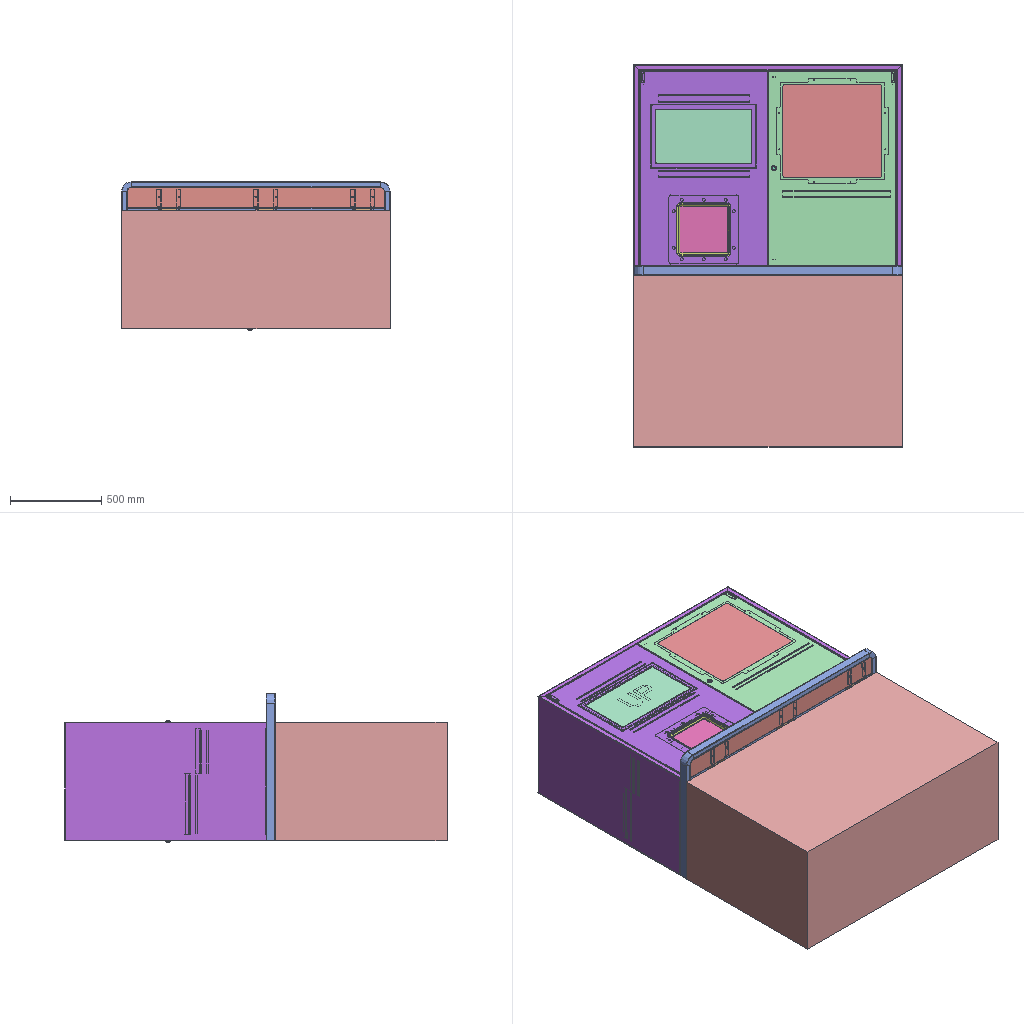Assembly | SolidWorks | 122 different items | 247 placed | box 1470 x 2090 x 812 mm
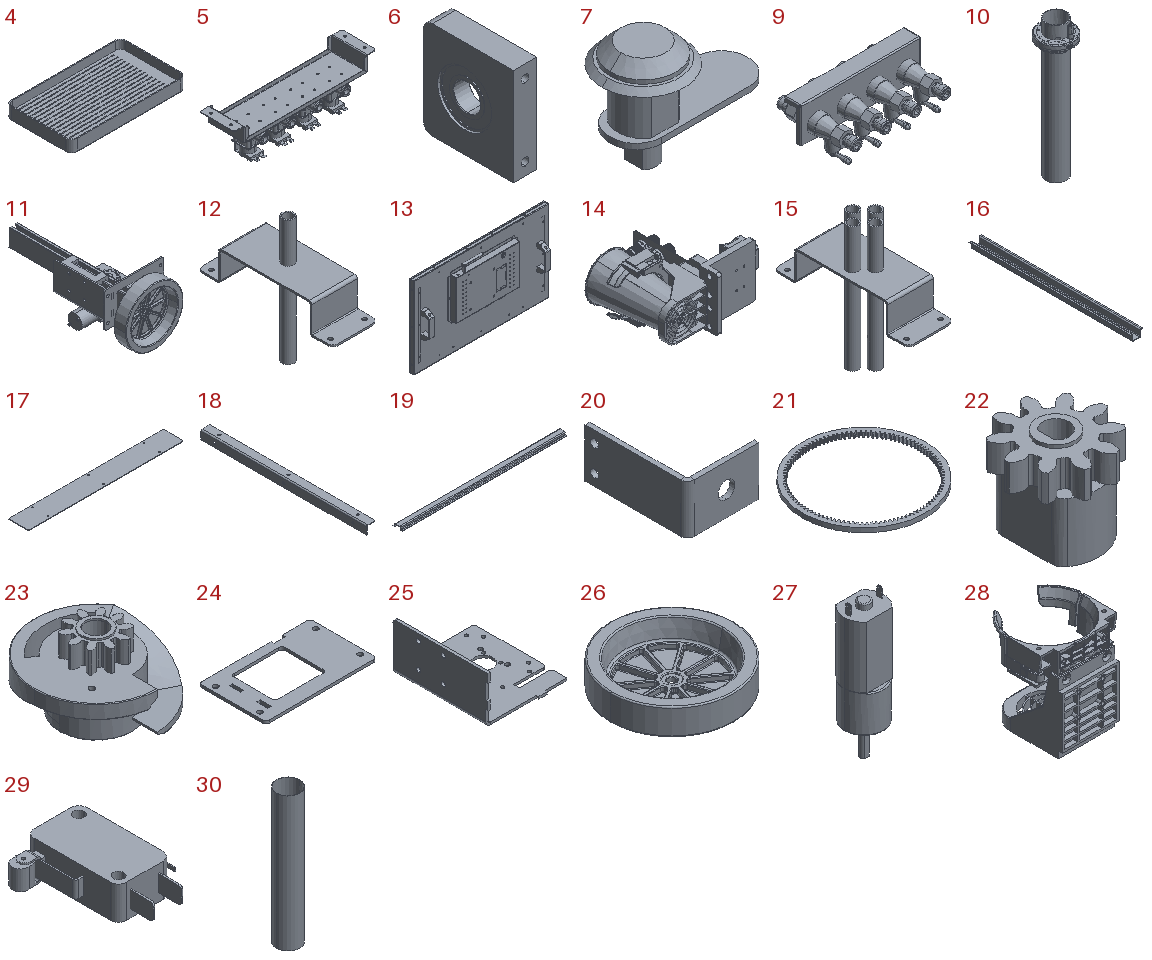Parts list (item | name | quantity | parent item | size | volume | features):
1 | 90 Capper Limit Switch Adjustable Bracket | x1 | - | - | - | -
2 | 90 mm Bore 5840-42 Rotary Capper Motor | x1 | - | - | - | -
3 | 90 mm Capper Limit Switch | x1 | - | - | - | -
4 | (subassembly) | x1 | - | 390 x 225 x 48 mm | 613615 mm3 | features AEMSimFeature 1
5 | (subassembly) | x1 | - | 287.6 x 73.8 x 84.7 mm | 205450 mm3 | features ReferencePattern 3, AEMSimFeature 1, LocalLPattern 1
6 | (subassembly) | x2 | in 14 | 13 x 50 x 54 mm | 29631 mm3 | features AEMSimFeature 1
7 | (subassembly) | x2 | - | 53.001 x 30 x 37.4 mm | 9862 mm3 | features AEMSimFeature 1
8 | (subassembly) | x1 | - | - | - | features AEMSimFeature 1
9 | (subassembly) | x1 | - | 222.4 x 141.4 x 82.578 mm | 275099 mm3 | features ReferencePattern 3, AEMSimFeature 1, LocalLPattern 1
10 | (subassembly) | x4 | - | - | 425730 mm3 | features InContextFeatHolder 5, ReferencePattern 4, LocalCirPattern 1
11 | (subassembly) | x1 | - | 115 x 241 x 107.2 mm | 279061 mm3 | features InContextFeatHolder 17
12 | (subassembly) | x1 | - | 40 x 119 x 110 mm | 12883 mm3 | features AEMSimFeature 1
13 | (subassembly) | x1 | - | 580.3 x 59 x 351.2 mm | 2110380 mm3 | features AEMSimFeature 1
14 | (subassembly) | x1 | in 8 | 224.692 x 193 x 105 mm | 423865 mm3 | features ReferencePattern 3, AEMSimFeature 1, InContextFeatHolder 1, LocalLPattern 1
15 | (subassembly) | x1 | - | 40 x 119 x 110 mm | 21860 mm3 | features LocalLPattern 2, ReferencePattern 2, AEMSimFeature 1
16 | - | x2 | - | 40 x 500 x 21 mm | 56565 mm3 | features 3DProfileFeature 1, FlatPattern 1, HoleWzd 1, ICE 1, SMBaseFlange 1, SheetMetal 1
17 | - | x2 | - | 500 x 65 x 1.5 mm | 48608 mm3 | features Fillet 1, FlatPattern 1, ICE 1, LPattern 1, SMBaseFlange 1, SheetMetal 1
18 | - | x2 | - | 30 x 575 x 30 mm | 64402 mm3 | features 3DProfileFeature 2, Fillet 2, HoleWzd 2, FlatPattern 1, ICE 1, LPattern 1, SMBaseFlange 1, SheetMetal 1
19 | - | x5 | - | 590 x 34 x 10.7 mm | 34971 mm3 | features EdgeFlange 2, FlatPattern 1, SMBaseFlange 1, SheetMetal 1
20 | - | x4 | - | 22 x 31.5 x 15 mm | 1109 mm3 | features ICE 2, FlatPattern 1, SMBaseFlange 1, SheetMetal 1
21 | - | x4 | in 10 | 144.5 x 144.5 x 5.2 mm | 14739 mm3 | features CirPattern 1, Extrusion 1, ICE 1, RefAxis 1
22 | - | x4 | in 10 | 15 x 14.473 x 13.6 mm | 1407 mm3 | features ICE 5, CirPattern 1, Extrusion 1, Fillet 1, RefAxis 1
23 | - | x20 | in 10 | 34.7 x 34.7 x 20.5 mm | 6291 mm3 | features ICE 12, Chamfer 4, Fillet 4, CirPattern 2, Helix 2, SweepCut 2, Extrusion 1, RefAxis 1
24 | - | x1 | in 11 | 100 x 60 x 2.5 mm | 10028 mm3 | features Cut 2, Fillet 2, ICE 2, MirrorPattern 2, FlatPattern 1, LPattern 1, SMBaseFlange 1, SheetMetal 1
25 | - | x1 | in 11 | 85 x 99.5 x 50 mm | 30184 mm3 | features Cut 4, Fillet 2, ICE 2, EdgeFlange 1, FlatPattern 1, LPattern 1, SMBaseFlange 1, SheetMetal 1
26 | - | x1 | in 11 | 98 x 98 x 21 mm | 76167 mm3 | features ICE 6, Fillet 5, Chamfer 2, CirPattern 1, Extrusion 1
27 | - | x4 | in 10 | 20.5 x 20 x 71.9 mm | 15341 mm3 | features ICE 8, Fillet 4, MirrorPattern 3, Extrusion 1
28 | - | x1 | in 14 | 95.114 x 93.076 x 111.7 mm | 101033 mm3 | features MBimport 1
29 | - | x4 | in 10 | 27.9 x 35 x 10 mm | 4554 mm3 | features ICE 3, BaseBody 1
30 | - | x4 | in 10 | 97 x 97 x 558.5 mm | 201706 mm3 | features Extrusion 1
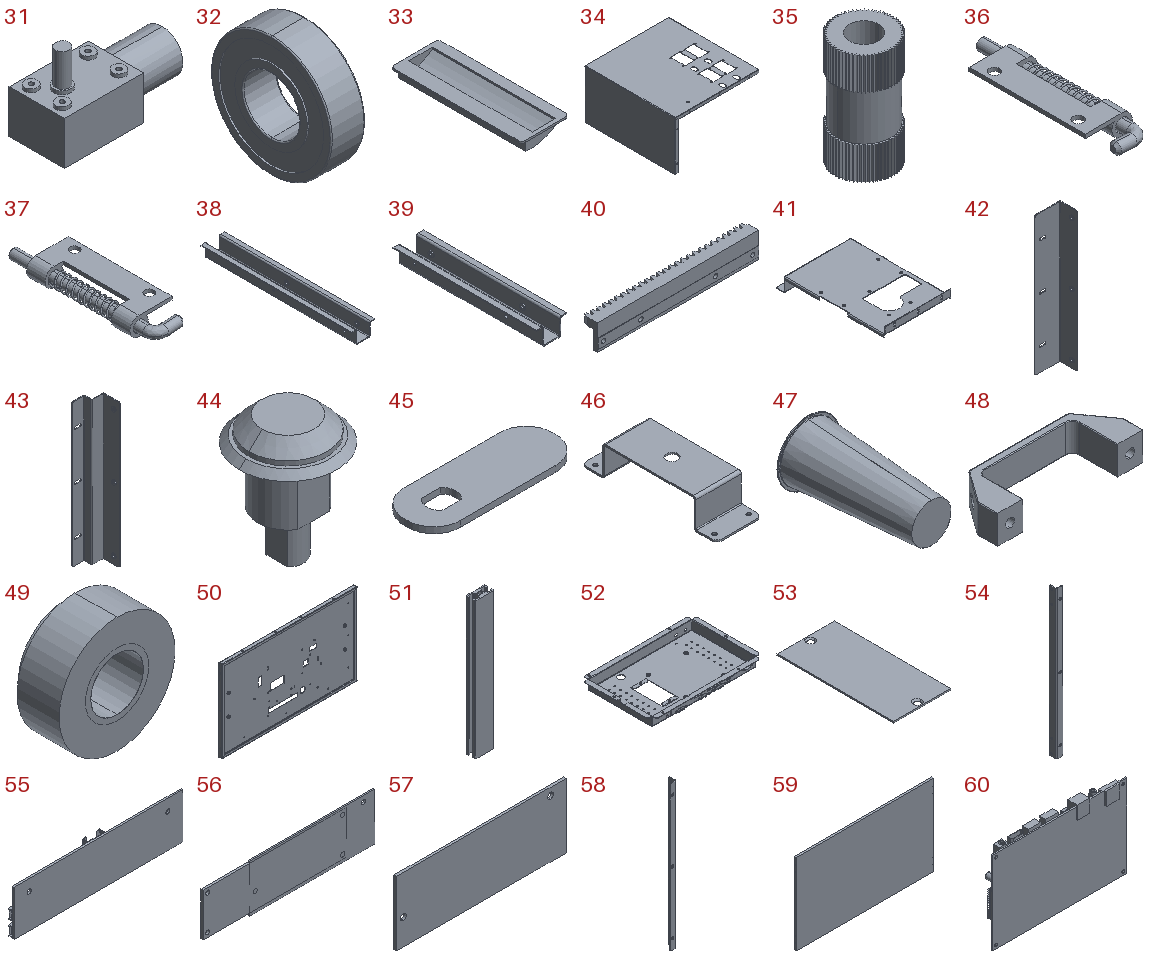31 | - | x1 | in 11 | 81 x 32 x 47.2 mm | 52588 mm3 | features ICE 7, Extrusion 1
32 | - | x2 | in 6 | 9 x 32 x 32 mm | 5366 mm3 | features BaseBody 1
33 | - | x2 | - | 40 x 110 x 10.429 mm | 7857 mm3 | features ICE 3, Extrusion 1, Fillet 1, MirrorPattern 1
34 | - | x1 | - | 568 x 611 x 333 mm | 859533 mm3 | features LPattern 4, ICE 3, Cut 2, EdgeFlange 2, 3DProfileFeature 1, FlatPattern 1, HoleWzd 1, SMBaseFlange 1, SheetMetal 1
35 | - | x16 | in 10 | 6.299 x 6.297 x 12 mm | 240.496 mm3 | features ICE 2, CirPattern 1, Extrusion 1
36 | - | x3 | - | 25.4 x 89 x 11 mm | 6004 mm3 | features MirrorStock 1
37 | - | x3 | - | 25.4 x 89 x 11 mm | 6004 mm3 | features BaseBody 3
38 | - | x2 | - | 50 x 320 x 28.5 mm | 48347 mm3 | features ICE 2, 3DProfileFeature 1, FlatPattern 1, HoleWzd 1, MirrorPattern 1, SMBaseFlange 1, SheetMetal 1
39 | - | x2 | - | 50 x 235 x 28.5 mm | 35580 mm3 | features ICE 2, 3DProfileFeature 1, FlatPattern 1, HoleWzd 1, MirrorPattern 1, SMBaseFlange 1, SheetMetal 1
40 | - | x1 | in 11 | 169.646 x 15.5 x 27 mm | 32516 mm3 | features ICE 4, LPattern 3, Boss 1, Chamfer 1, Extrusion 1, Fillet 1
41 | - | x1 | - | 236 x 382 x 73.5 mm | 191072 mm3 | features ICE 7, EdgeFlange 4, Fillet 2, SMBaseFlange 2, FlatPattern 1, MirrorPattern 1, SheetMetal 1
42 | - | x1 | - | 50 x 35 x 270 mm | 33491 mm3 | features ICE 2, 3DProfileFeature 1, Fillet 1, FlatPattern 1, HoleWzd 1, SMBaseFlange 1, SheetMetal 1
43 | - | x1 | - | 45 x 47 x 270 mm | 35809 mm3 | features ICE 2, 3DProfileFeature 1, Fillet 1, FlatPattern 1, HoleWzd 1, SMBaseFlange 1, SheetMetal 1
44 | - | x2 | in 7 | 30 x 30 x 37.4 mm | 8223 mm3 | features ICE 3, Chamfer 2, Extrusion 1
45 | - | x2 | in 7 | 50 x 19 x 2 mm | 1640 mm3 | features Fillet 1, FlatPattern 1, ICE 1, SMBaseFlange 1, SheetMetal 1
46 | - | x1 | in 12 | 40 x 119 x 26.5 mm | 9773 mm3 | features EdgeFlange 2, ICE 2, Fillet 1, FlatPattern 1, LPattern 1, SMBaseFlange 1, SheetMetal 1
47 | - | x1 | in 14 | 89 x 177.3 x 89 mm | 12581 mm3 | features RefAxis 1, Revolution 1
48 | - | x2 | in 13 | 107.5 x 38 x 21 mm | 27579 mm3 | features BaseBody 1
49 | - | x1 | in 13 | - | - | features BaseBody 1, RefSurface 1
50 | - | x1 | in 13 | - | - | features BaseBody 13, RefSurface 1
51 | - | x1 | in 11 | 30 x 15 x 220 mm | 49057 mm3 | features ICE 4, Fillet 2, MirrorPattern 2, Cut 1, Extrusion 1, LPattern 1
52 | - | x1 | in 13 | - | - | features RefSurface 13, BaseBody 12
53 | - | x1 | in 13 | 41 x 84 x 1 mm | 3404 mm3 | features BaseBody 1
54 | - | x1 | in 13 | 12 x 14.1 x 280 mm | 6830 mm3 | features BaseBody 1
55 | - | x1 | in 13 | 134 x 11.5 x 36 mm | 18226 mm3 | features BaseBody 1
56 | - | x1 | in 13 | 119.5 x 1.6 x 33.1 mm | 8199 mm3 | features BaseBody 2
57 | - | x1 | in 13 | 87 x 1.2 x 33.1 mm | 3439 mm3 | features BaseBody 1
58 | - | x1 | in 13 | 12 x 14.1 x 280 mm | 6824 mm3 | features BaseBody 1
59 | - | x1 | in 13 | 545 x 7.9 x 320.7 mm | 1351854 mm3 | features BaseBody 1
60 | - | x1 | in 13 | 154 x 11.8 x 97.6 mm | 32495 mm3 | features BaseBody 5
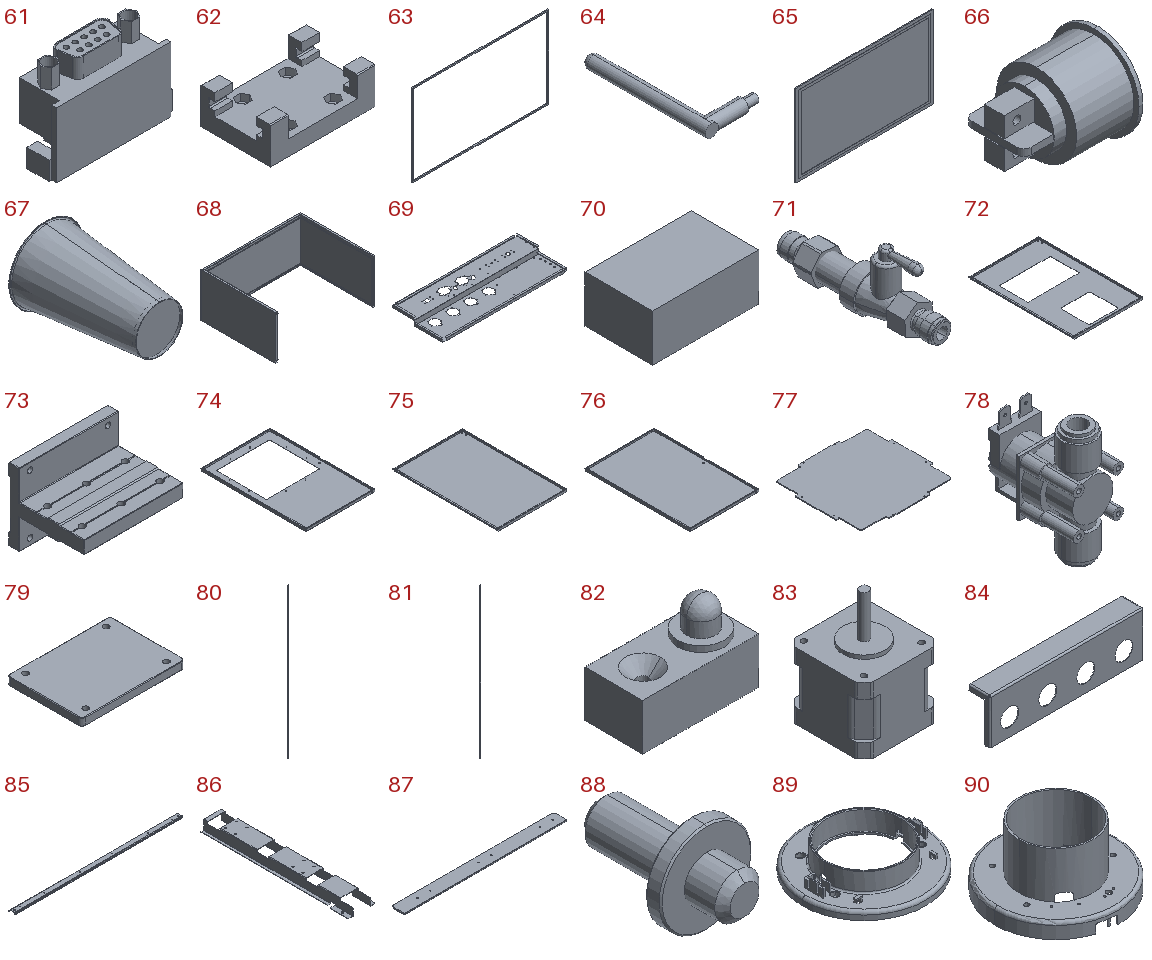61 | - | x1 | in 13 | 38.5 x 14 x 26.3 mm | 7123 mm3 | features BaseBody 1
62 | - | x1 | in 11 | 60 x 40 x 21 mm | 23831 mm3 | features ICE 6, MirrorPattern 5, Chamfer 1, Extrusion 1
63 | - | x1 | in 13 | 579 x 4.5 x 350 mm | 41355 mm3 | features BaseBody 1
64 | - | x1 | in 13 | 39.5 x 87.5 x 9.5 mm | 7324 mm3 | features BaseBody 1
65 | - | x1 | in 13 | 569 x 4.9 x 340 mm | 738758 mm3 | features BaseBody 1
66 | - | x1 | in 13 | 23 x 18 x 18 mm | 3351 mm3 | features BaseBody 1
67 | - | x1 | in 14 | 88.983 x 137.24 x 88.983 mm | 20015 mm3 | features Revolution 1
68 | - | x1 | - | 1470 x 1100 x 650 mm | 4400444 mm3 | features EdgeFlange 6, MirrorPattern 3, 3DProfileFeature 1, Cut 1, FlatPattern 1, HoleWzd 1, ICE 1, LPattern 1, SMBaseFlange 1, SheetMetal 1
69 | - | x1 | - | 1460 x 594.237 x 88.5 mm | 1606970 mm3 | features ICE 14, Cut 9, EdgeFlange 7, LPattern 7, Fillet 6, 3DProfileFeature 5, HoleWzd 5, Chamfer 1, FlatPattern 1, SMBaseFlange 1, SheetMetal 1
70 | - | x1 | - | 1470 x 940 x 650 mm | 898157138 mm3 | features Extrusion 1, ICE 1
71 | - | x4 | in 9 | 33.3 x 141.4 x 59.55 mm | 62869 mm3 | features BaseBody 3
72 | - | x1 | - | 713.5 x 1066 x 27.237 mm | 927429 mm3 | features Fillet 4, Cut 3, EdgeFlange 3, ICE 3, FlatPattern 1, LPattern 1, SMBaseFlange 1, SheetMetal 1
73 | - | x2 | - | 92 x 70 x 67 mm | 123331 mm3 | features MBimport 1
74 | - | x1 | - | 700 x 1066 x 25 mm | 867025 mm3 | features ICE 8, Fillet 3, EdgeFlange 2, Cut 1, FlatPattern 1, LPattern 1, MirrorPattern 1, SMBaseFlange 1, SheetMetal 1
75 | - | x1 | - | 713.5 x 1066 x 27.237 mm | 1292655 mm3 | features EdgeFlange 3, ICE 3, Fillet 1, FlatPattern 1, LPattern 1, SMBaseFlange 1, SheetMetal 1
76 | - | x1 | - | 700 x 1066 x 25 mm | 1278991 mm3 | features Cut 4, EdgeFlange 2, ICE 2, Fillet 1, FlatPattern 1, LPattern 1, MirrorPattern 1, SMBaseFlange 1, SheetMetal 1
77 | - | x1 | - | 610 x 575 x 5 mm | 1627713 mm3 | features Fillet 2, ICE 2, Extrusion 1
78 | - | x4 | in 5 | 34 x 54.7 x 70 mm | 42821 mm3 | features MBimport 1
79 | - | x2 | - | 92 x 67 x 7 mm | 42466 mm3 | features Chamfer 1, Extrusion 1, Fillet 1, ICE 1, LPattern 1
80 | - | x2 | - | 10 x 6 x 1410 mm | 19879 mm3 | features Extrusion 1
81 | - | x4 | - | 10 x 6 x 1058 mm | 14916 mm3 | features Extrusion 1
82 | - | x8 | in 10 | 20 x 10 x 14 mm | 1686 mm3 | features ICE 3, Chamfer 1, Extrusion 1, Fillet 1
83 | - | x1 | in 14 | 41.6 x 41.6 x 60.7 mm | 59288 mm3 | features ICE 2, MBimport 1
84 | - | x1 | in 9 | 222.4 x 30 x 65 mm | 23557 mm3 | features EdgeFlange 6, Fillet 4, ICE 3, LPattern 2, SMBaseFlange 2, Cut 1, FlatPattern 1, SheetMetal 1
85 | - | x4 | - | 1410 x 53 x 13 mm | 143996 mm3 | features EdgeFlange 2, MirrorPattern 2, 3DProfileFeature 1, Cut 1, FlatPattern 1, HoleWzd 1, ICE 1, SMBaseFlange 1, SheetMetal 1
86 | - | x3 | - | 132 x 730 x 48.5 mm | 188452 mm3 | features ICE 5, EdgeFlange 3, LPattern 3, 3DProfileFeature 2, Fillet 2, HoleWzd 2, SMBaseFlange 2, FlatPattern 1, MirrorPattern 1, SheetMetal 1
87 | - | x1 | - | 1408 x 114.6 x 10 mm | 275844 mm3 | features 3DProfileFeature 1, EdgeFlange 1, Fillet 1, FlatPattern 1, HoleWzd 1, LPattern 1, SMBaseFlange 1, SheetMetal 1
88 | - | x6 | - | 12 x 19 x 12 mm | 657.73 mm3 | features BaseBody 1
89 | - | x4 | in 10 | 160 x 160 x 38 mm | 58176 mm3 | features ICE 18, Fillet 7, Chamfer 2, CirPattern 2, Cut 1, Extrusion 1, MirrorPattern 1
90 | - | x4 | in 10 | 160 x 160 x 88 mm | 94016 mm3 | features ICE 20, CirPattern 4, Fillet 4, Chamfer 2, Cut 1, DelFace 1, Extrusion 1
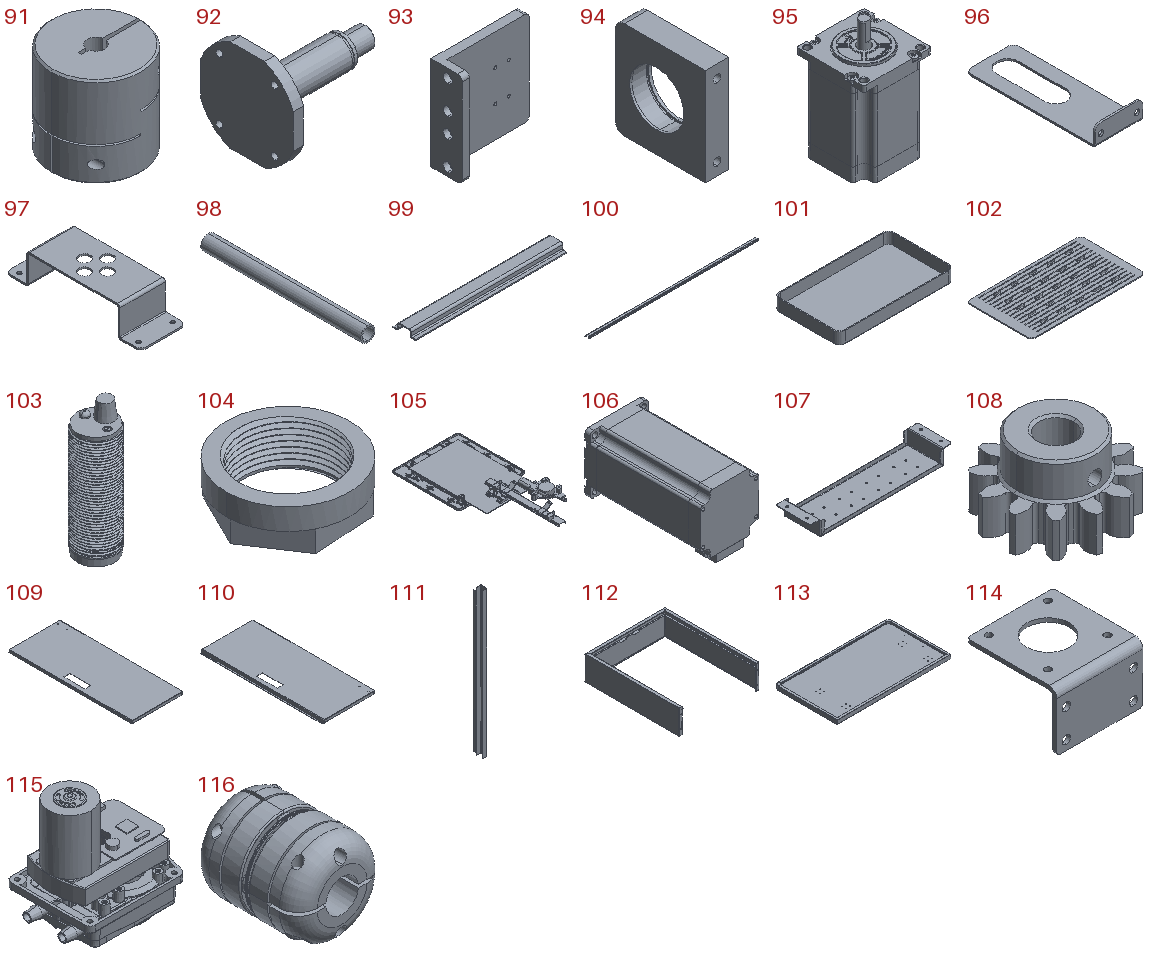91 | - | x1 | in 14 | 26 x 26 x 26 mm | 11774 mm3 | features ICE 6, RevCut 2, Chamfer 1, Extrusion 1
92 | - | x1 | in 14 | 58 x 45 x 45 mm | 17000 mm3 | features 3DProfileFeature 1, Chamfer 1, HoleWzd 1, ICE 1, RevCut 1, Revolution 1
93 | - | x1 | in 14 | 100 x 35 x 105 mm | 123455 mm3 | features ICE 5, 3DProfileFeature 2, Fillet 2, HoleWzd 2, ExtruThin 1
94 | - | x2 | in 6 | 13 x 50 x 54 mm | 23974 mm3 | features ICE 4, 3DProfileFeature 2, HoleWzd 2, ExtruThin 1, Fillet 1, RevCut 1
95 | - | x1 | in 8 | - | - | features RefSurface 16, BaseBody 14
96 | - | x1 | in 14 | 40 x 108 x 16 mm | 5776 mm3 | features ICE 2, EdgeFlange 1, Fillet 1, FlatPattern 1, SMBaseFlange 1, SheetMetal 1
97 | - | x1 | in 15 | 40 x 119 x 26.5 mm | 9419 mm3 | features EdgeFlange 2, ICE 2, Fillet 1, FlatPattern 1, LPattern 1, RefAxis 1, SMBaseFlange 1, SheetMetal 1
98 | - | x5 | in 12, 15 | 10 x 110 x 10 mm | 3110 mm3 | features Sweep 1
99 | - | x3 | - | 230 x 34 x 11 mm | 16952 mm3 | features EdgeFlange 2, FlatPattern 1, SMBaseFlange 1, SheetMetal 1
100 | - | x1 | - | 1375 x 34 x 11 mm | 101345 mm3 | features EdgeFlange 2, FlatPattern 1, SMBaseFlange 1, SheetMetal 1
101 | - | x1 | in 4 | 390 x 225 x 48 mm | 398371 mm3 | features Fillet 3, Extrusion 1, ICE 1, LPattern 1, Shell 1
102 | - | x1 | in 4 | 384 x 219 x 9 mm | 215244 mm3 | features ICE 2, LPattern 2, Extrusion 1, Fillet 1
103 | - | x2 | in 14 | 17.6 x 17.6 x 57.2 mm | 11322 mm3 | features MBimport 1
104 | - | x4 | in 14 | 23 x 23 x 8 mm | 1078 mm3 | features MBimport 1
105 | - | x1 | - | 380 x 785.607 x 83.5 mm | 1277460 mm3 | features BaseBody 24, RefSurface 1
106 | - | x1 | in 8 | 56.4 x 132.5 x 68.6 mm | 185240 mm3 | features BaseBody 11
107 | - | x1 | in 5 | 287.6 x 73.8 x 30 mm | 34168 mm3 | features EdgeFlange 3, Fillet 3, LPattern 2, Cut 1, FlatPattern 1, ICE 1, SMBaseFlange 1, SheetMetal 1
108 | - | x1 | in 11 | 27.338 x 27.338 x 16 mm | 4690 mm3 | features ICE 5, Chamfer 2, CirPattern 1, Extrusion 1, RefAxis 1
109 | - | x1 | - | 257 x 620 x 14 mm | 226694 mm3 | features EdgeFlange 2, ICE 2, SMBaseFlange 2, Cut 1, Fillet 1, FlatPattern 1, LPattern 1, SheetMetal 1
110 | - | x1 | - | 264.8 x 620 x 16 mm | 228976 mm3 | features EdgeFlange 4, Fillet 2, ICE 2, SMBaseFlange 2, Cut 1, FlatPattern 1, LPattern 1, SheetMetal 1
111 | - | x1 | - | 19.1 x 31.2 x 525 mm | 39715 mm3 | features EdgeFlange 1, FlatPattern 1, SMBaseFlange 1, SheetMetal 1
112 | - | x1 | - | 568.4 x 668.4 x 173.4 mm | 516143 mm3 | features EdgeFlange 5, ICE 3, Fillet 2, SMBaseFlange 2, Cut 1, FlatPattern 1, MirrorPattern 1, SheetMetal 1
113 | - | x1 | - | 1469 x 804.6 x 50 mm | 2339637 mm3 | features EdgeFlange 11, 3DProfileFeature 4, Cut 3, LPattern 3, MirrorPattern 2, Fillet 1, FlatPattern 1, SMBaseFlange 1, SheetMetal 1
114 | - | x1 | in 14 | 45 x 47 x 30 mm | 5671 mm3 | features 3DProfileFeature 2, HoleWzd 2, EdgeFlange 1, Fillet 1, FlatPattern 1, ICE 1, SMBaseFlange 1, SheetMetal 1
115 | - | x4 | - | 110.761 x 88 x 135.55 mm | 287253 mm3 | features BaseBody 6
116 | - | x2 | in 8 | 32.5 x 40 x 32.5 mm | 24280 mm3 | features BaseBody 23
117 | circlips for holes--type a gb | x1 | - | - | - | -
118 | circlips for shaft--type a large gb | x1 | - | - | - | -
119 |  Capper Welded Bracket | x1 | - | - | - | -
120 |  Capper Limit Switch Bracket | x1 | - | - | - | -
121 |  Capper Limit Spring Leaf | x1 | - | - | - | -
122 |  Adjustable Profile Switch Bracket Drill Hole Fixture | x1 | - | - | - | -
Mates (type | each side: item.copy, entity, surface, feature):
In the top assembly
Coincident | 70.1 face plane Boss-Extrude 1 | 113.1 face plane Edge-Flange 1 | 2 times
Coincident | 70.1 face plane Boss-Extrude 1 | 113.1 face plane Edge-Flange 2
Coincident | 74.1 face plane Base-Flange 1 | 77.1 face plane Boss-Extrude 1
Coincident | 113.1 face plane Base-Flange 1 | 85.1 face plane Edge-Flange 2
Width | 85.1 face plane Edge Bend 1 | 85.1 face plane Edge Bend 1 | 113.1 face plane Edge-Flange 1 | 113.1 face plane Edge-Flange 1
DistanceDim | 85.1 face plane Edge-Flange 1 | 113.1 face plane Edge-Flange 1
Coincident | 113.1 face plane Base-Flange 1 | 85.2 face plane Edge-Flange 2
Coincident | 85.3 face plane Edge-Flange 2 | 85.4 face plane Edge-Flange 2
Coincident | 85.2 face plane Edge-Flange 2 | 85.4 face plane Edge-Flange 2
Coincident | 85.1 face plane Edge Bend 4 | 85.2 face plane Edge Bend 4
Coincident | 85.2 face plane Base-Flange 1 | 85.4 face plane Base-Flange 1
Coincident | 85.3 face plane Edge Bend 4 | 85.4 face plane Edge-Flange 2
DistanceDim | 85.3 face plane Edge-Flange 1 | 85.4 face plane Edge-Flange 1
DistanceDim | 85.4 face plane Edge-Flange 1 | 85.2 face plane Edge-Flange 1
Coincident | 113.1 face plane Base-Flange 1 | 68.1 face plane Edge-Flange 4
Coincident | 113.1 face plane Edge-Flange 1 | 68.1 face plane Edge-Flange 1
Coincident | 113.1 face plane Edge-Flange 1 | 68.1 face plane Base-Flange 1
Coincident | 113.1 face plane Base-Flange 1 | 18.1 face plane Base-Flange 1
Coincident | 68.1 face plane Edge-Flange 5 | 18.1 face plane Base-Flange 1
Coincident | 113.1 face plane Edge-Flange 2 | 87.1 face plane Edge-Flange 1
Width | 77.1 face plane Boss-Extrude 1 | 77.1 face plane Boss-Extrude 1 | 74.1 face plane Cut-Extrude 1 | 74.1 face plane Boss-Extrude 1
Width | 77.1 face plane Boss-Extrude 1 | 77.1 face plane Boss-Extrude 1 | 74.1 face plane Cut-Extrude 1 | 74.1 face plane Cut-Extrude 1
Coincident | 65.1 face plane Import 1 | 72.1 face plane Base-Flange 1
Parallel | 50.1 face plane Curved Face-Import 4 | 72.1 face plane Edge-Flange 1
Width | 65.1 face plane Import 1 | 65.1 face plane Import 1 | 72.1 face plane Cut-Extrude 1 | 72.1 face plane Cut-Extrude 1 | 2 times
Parallel | 68.1 face plane Base-Flange 1 | 105.1 face plane
Coincident | 72.1 face plane Base-Flange 1 | 16.1 face plane Base-Flange 1
Parallel | 50.1 face plane Curved Face-Import 4 | 16.1 face plane Base-Flange 1
Coincident | 72.1 face plane Base-Flange 1 | 16.2 face plane Base-Flange 1
Coincident | 16.1 face plane Base-Flange 1 | 16.2 face plane Base-Flange 1
Coincident | 50.1 face plane Curved Face-Import 4 | 17.1 face plane Base-Flange 1
Concentric | 50.1 face cylinder Curved Face-Import 4 | 17.1 face cylinder LPattern 1
Parallel | 50.1 face plane Curved Face-Import 4 | 17.1 face plane Base-Flange 1
Concentric | 16.1 face cylinder M4 Tapped Hole 1 | 17.1 face cylinder Cut-Extrude 1
Parallel | 16.1 face plane Base-Flange 1 | 17.1 face plane Base-Flange 1
Coincident | 16.2 face plane Base-Flange 1 | 17.2 face plane Base-Flange 1
Concentric | 50.1 face cylinder Curved Face-Import 4 | 17.2 face cylinder Cut-Extrude 1
Parallel | 50.1 face plane Curved Face-Import 4 | 17.2 face plane Base-Flange 1
Concentric | 16.2 face cylinder M4 Tapped Hole 1 | 17.2 face cylinder LPattern 1
Parallel | 16.2 face plane Base-Flange 1 | 17.2 face plane Base-Flange 1
Coincident | 68.1 face plane Base-Flange 1 | 38.1 face plane Base-Flange 1
Parallel | 34.1 face plane Edge-Flange 2 | 115.1 face plane Peristaltic Pump 304k.STEP-1/JIETOU.STEP-1-solid1
Coincident | 34.1 face plane Base-Flange 1 | 115.1 face plane Peristaltic Pump 304k.STEP-1/23_3_26_.STEP-1-solid1
Coincident | 68.1 face plane Edge-Flange 5 | 18.2 face plane Base-Flange 1
Coincident | 113.1 face plane Base-Flange 1 | 18.2 face plane Base-Flange 1
Concentric | 34.1 face cylinder LPattern 2 | 115.1 face cylinder Peristaltic Pump 304k.STEP-1/23_3_26_.STEP-1-solid1
DistanceDim | 38.1 face plane Base-Flange 1 | 68.1 face plane Edge-Flange 4
DistanceDim | 68.1 face plane Edge-Flange 5 | 18.1 face plane Cut-Extrude 1
DistanceDim | 68.1 face plane Edge-Flange 5 | 18.2 face plane Cut-Extrude 1
Coincident | 113.1 face plane Base-Flange 1 | 43.1 face plane Base-Flange 1
Coincident | 105.1 face plane | 43.1 face plane Base-Flange 1
Width | 105.1 face plane | 105.1 face plane | 43.1 face plane Base-Flange 1 | 43.1 face plane Base-Flange 1
Coincident | 34.1 face plane Edge-Flange 1 | 112.1 face plane Base-Flange 1
Coincident | 34.1 face plane Base-Flange 1 | 112.1 face plane Edge-Flange 1
Concentric | 112.1 face cylinder Cut-Extrude 3 | 109.1 face cylinder Cut-Extrude 1
Concentric | 109.1 face cylinder Cut-Extrude 1 | 88.1 face cylinder Import 1
Coincident | 109.1 face plane Edge-Flange 1 | 88.1 face plane Import 1
Concentric | 88.2 face cylinder Import 1 | 110.1 face cylinder Cut-Extrude 1
Coincident | 88.2 face plane Import 1 | 110.1 face plane Edge-Flange 1
Coincident | 105.1 face plane Electric Lift DoorAssembly with Sheet Metal Bracket 5(1).STEP-1/KFJ-01.STEP-1/CH-1_.STEP-1-solid1 | 41.1 face plane Base-Flange 1
Concentric | 105.1 face cylinder Electric Lift DoorAssembly with Sheet Metal Bracket 5(1).STEP-1/KFJ-01.STEP-1/CH-1_.STEP-1-solid1 | 41.1 face cylinder Cut-Extrude 1 | 2 times
Coincident | 75.1 face plane Base-Flange 1 | 37.1 face plane Gen3 MANIFOLD_SOLID_BREP_8333_21-1-solid1
Parallel | 75.1 face plane Edge-Flange 1 | 37.1 face plane Gen3 MANIFOLD_SOLID_BREP_8333_21-1-solid1
Concentric | 75.1 face cylinder Cut-Extrude 2 | 88.3 face cylinder Import 1
Coincident | 75.1 face plane Edge-Flange 1 | 88.3 face plane Import 1
Concentric | 75.1 face cylinder Boss-Extrude 1 | 37.1 face cylinder Gen3 MANIFOLD_SOLID_BREP_8333_21-1-solid1
Coincident | 113.1 face plane Base-Flange 1 | 88.3 face plane Import 1
Concentric | 68.1 face cylinder Cut-Extrude 1 | 37.1 face cylinder Gen3 MANIFOLD_SOLID_BREP_8623_21-1-solid1
Coincident | 76.1 face plane Edge-Flange 1 | 75.1 face plane Edge-Flange 1
Concentric | 76.1 face cylinder Cut-Extrude 1 | 88.4 face cylinder Import 1
Coincident | 76.1 face plane Edge-Flange 1 | 88.4 face plane Import 1
Coincident | 76.1 face plane Base-Flange 1 | 36.1 face plane
Concentric | 76.1 face cylinder Boss-Extrude 1 | 36.1 face cylinder
Concentric | 76.1 face cylinder LPattern 1 | 36.1 face cylinder
Concentric | 68.1 face cylinder Mirror 2 | 36.1 face cylinder
Coincident | 70.1 face plane Boss-Extrude 1 | 75.1 face plane Base-Flange 1
Coincident | 76.1 face plane Base-Flange 1 | 44.1 face plane Boss-Extrude 4
Concentric | 76.1 face cylinder Cut-Extrude 2 | 44.1 face cylinder Boss-Extrude 2
Parallel | 44.1 face plane Boss-Extrude 2 | 76.1 face plane Edge-Flange 1
Coincident | 74.1 face plane Base-Flange 1 | 36.2 face plane
Parallel | 74.1 face plane Edge-Flange 1 | 36.2 face plane
Concentric | 74.1 face cylinder LPattern 1 | 36.2 face cylinder
Concentric | 74.1 face cylinder Cut-Extrude 3 | 88.5 face cylinder Import 1
Coincident | 74.1 face plane Edge-Flange 1 | 88.5 face plane Import 1
Concentric | 68.1 face cylinder Mirror 3 | 36.2 face cylinder
Coincident | 113.1 face plane Base-Flange 1 | 88.5 face plane Import 1
Coincident | 72.1 face plane Base-Flange 1 | 37.2 face plane Gen3 MANIFOLD_SOLID_BREP_8333_21-1-solid1
Concentric | 72.1 face cylinder Boss-Extrude 1 | 37.2 face cylinder Gen3 MANIFOLD_SOLID_BREP_8333_21-1-solid1
Concentric | 72.1 face cylinder LPattern 1 | 37.2 face cylinder Gen3 MANIFOLD_SOLID_BREP_8333_21-1-solid1
Concentric | 72.1 face cylinder Cut-Extrude 4 | 88.6 face cylinder Import 1
Coincident | 72.1 face plane Edge-Flange 1 | 88.6 face plane Import 1
Coincident | 113.1 face plane Base-Flange 1 | 88.6 face plane Import 1
Concentric | 68.1 face cylinder Mirror 3 | 37.2 face cylinder Gen3 MANIFOLD_SOLID_BREP_8623_21-1-solid1
DistanceDim | 105.1 face plane | 113.1 face plane Edge-Flange 1
DistanceDim | 105.1 face plane | 113.1 face plane Base-Flange 1
Coincident | 105.1 face plane | 42.1 face plane Base-Flange 1
Coincident | 74.1 face plane Base-Flange 1 | 44.2 face plane Boss-Extrude 4
Concentric | 74.1 face cylinder Cut-Extrude 4 | 44.2 face cylinder Boss-Extrude 2
DistanceDim | 113.1 face plane Base-Flange 1 | 101.1 face plane LPattern 1
Coincident | 112.1 face plane Edge-Flange 2 | 111.1 face plane Base-Flange 1
Coincident | 112.1 face plane Base-Flange 1 | 111.1 face plane Base-Flange 1
Coincident | 112.1 face plane Edge-Flange 3 | 111.1 face plane Base-Flange 1
Coincident | 88.2 face plane Import 1 | 111.1 face plane Base-Flange 1
Concentric | 112.1 face cylinder Mirror 1 | 110.1 face cylinder Cut-Extrude 1
Coincident | 110.1 face plane Base-Flange 1 | 37.3 face plane Gen3 MANIFOLD_SOLID_BREP_8333_21-1-solid1
Concentric | 110.1 face cylinder Boss-Extrude 1 | 37.3 face cylinder Gen3 MANIFOLD_SOLID_BREP_8333_21-1-solid1
Concentric | 110.1 face cylinder LPattern 1 | 37.3 face cylinder Gen3 MANIFOLD_SOLID_BREP_8333_21-1-solid1
Coincident | 109.1 face plane Base-Flange 1 | 36.3 face plane
Concentric | 109.1 face cylinder Boss-Extrude 1 | 36.3 face cylinder
Concentric | 109.1 face cylinder LPattern 1 | 36.3 face cylinder
Coincident | 38.1 face plane Base-Flange 1 | 39.1 face plane Base-Flange 1
Coincident | 76.1 face plane Base-Flange 1 | 20.1 face plane Base-Flange 1
Concentric | 76.1 face cylinder Cut-Extrude 4 | 20.1 face cylinder Cut-Extrude 2 | 2 times
Coincident | 76.1 face plane Base-Flange 1 | 20.2 face plane Base-Flange 1
Concentric | 76.1 face cylinder Mirror 1 | 20.2 face cylinder Cut-Extrude 2 | 2 times
Perpendicular | 74.1 face plane Edge-Flange 1 | 44.2 face plane Boss-Extrude 2
Coincident | 74.1 face plane Base-Flange 1 | 20.3 face plane Base-Flange 1
Concentric | 74.1 face cylinder Cut-Extrude 6 | 20.3 face cylinder Cut-Extrude 2 | 2 times
Coincident | 74.1 face plane Base-Flange 1 | 20.4 face plane Base-Flange 1
Concentric | 74.1 face cylinder Mirror 1 | 20.4 face cylinder Cut-Extrude 2 | 2 times
Coincident | 76.1 face plane Base-Flange 1 | 75.1 face plane Base-Flange 1
Coincident | 69.1 face plane Base-Flange 1 | 100.1 face plane Edge-Flange 2
Coincident | 68.1 face plane Base-Flange 1 | 39.2 face plane Base-Flange 1
Coincident | 39.1 face plane Cut-Extrude 1 | 39.2 face plane Base-Flange 1
Coincident | 68.1 face plane Base-Flange 1 | 38.2 face plane Base-Flange 1
Coincident | 69.1 face plane Edge-Flange 3 | 38.2 face plane Base-Flange 1
Coincident | 38.1 face plane Base-Flange 1 | 38.2 face plane Cut-Extrude 1
DistanceDim | 38.1 face plane Base-Flange 1 | 68.1 face plane Edge-Flange 1
Coincident | 38.1 face plane Base-Flange 1 | 69.1 face plane Edge-Flange 3
DistanceDim | 69.1 face plane Edge-Flange 1 | 38.1 face plane Base-Flange 1
DistanceDim | 38.1 face plane Cut-Extrude 1 | 39.1 face plane Cut-Extrude 1
DistanceDim | 38.1 face plane Base-Flange 1 | 39.1 face plane Base-Flange 1
Coincident | 39.1 face plane Base-Flange 1 | 39.2 face plane Base-Flange 1
Parallel | 74.1 face plane Base-Flange 1 | 69.1 face plane Edge-Flange 12
Coincident | 72.1 face plane Base-Flange 1 | 74.1 face plane Base-Flange 1
Coincident | 68.1 face plane Edge-Flange 3 | 80.1 face plane Boss-Extrude 1 | 2 times
Coincident | 68.1 face plane Edge-Flange 2 | 80.1 face plane Boss-Extrude 1
Coincident | 68.1 face plane Edge-Flange 3 | 81.1 face plane Boss-Extrude 1 | 2 times
Coincident | 68.1 edge | 81.1 face plane Boss-Extrude 1
Coincident | 68.1 face plane Edge-Flange 3 | 81.2 face plane Boss-Extrude 1 | 2 times
Coincident | 68.1 edge | 81.2 face plane Boss-Extrude 1
DistanceDim | 68.1 face plane Edge-Flange 1 | 69.1 face plane Edge-Flange 1
Coincident | 75.1 face plane Base-Flange 1 | 19.1 face plane Edge-Flange 2
DistanceDim | 19.1 face plane Edge-Flange 1 | 75.1 face plane Edge-Flange 1
DistanceDim | 19.1 face plane Base-Flange 1 | 75.1 face plane Edge-Flange 1
Coincident | 76.1 face plane Base-Flange 1 | 19.2 face plane Edge-Flange 2
DistanceDim | 19.2 face plane Edge-Flange 1 | 76.1 face plane Edge-Flange 1
DistanceDim | 76.1 face plane Edge-Flange 1 | 19.2 face plane Edge-Flange 1
Coincident | 74.1 face plane Base-Flange 1 | 19.3 face plane Edge-Flange 2
DistanceDim | 19.3 face plane Base-Flange 1 | 74.1 face plane Edge-Flange 1
DistanceDim | 19.3 face plane Edge-Flange 1 | 74.1 face plane Edge-Flange 1
Coincident | 113.1 face plane Edge-Flange 2 | 87.1 face plane Base-Flange 1
Coincident | 113.1 face plane Base-Flange 1 | 86.1 face plane Base-Flange 1
Parallel | 113.1 face plane Edge-Flange 1 | 86.1 face plane Edge-Flange 1
Width | 113.1 face plane Edge-Flange 15 | 113.1 face plane Edge-Flange 14 | 87.1 face plane Edge-Flange 1 | 87.1 face plane Edge-Flange 1
Coincident | 34.1 face plane Edge-Flange 2 | 69.1 face plane Base-Flange 1
Coincident | 34.1 face plane Edge-Flange 2 | 69.1 face plane Edge-Flange 2
Coincident | 34.1 face plane Base-Flange 1 | 69.1 face plane Edge-Flange 10
Coincident | 46.1 face plane Edge-Flange 2 | 69.1 face plane Edge-Flange 11
Concentric | 98.1 face cylinder Sweep 1 | 69.1 face cylinder Cut-Extrude 19
Coincident | 69.1 face plane Edge-Flange 11 | 97.1 face plane Edge-Flange 2
Concentric | 69.1 face cylinder Cut-Extrude 19 | 97.1 axis
Coincident | 41.1 face plane Edge-Flange 7 | 69.1 face plane Edge-Flange 12
Parallel | 42.1 face plane Base-Flange 1 | 69.1 face plane Edge-Flange 11
Concentric | 105.1 face cylinder | 42.1 face cylinder M4 Tapped Hole 1
Parallel | 34.1 face plane Edge-Flange 2 | 107.1 face plane Edge-Flange 3
Coincident | 34.1 face plane Base-Flange 1 | 84.1 face plane Edge-Flange 4
Parallel | 107.1 face plane Edge-Flange 3 | 84.1 face plane Edge-Flange 5
Coincident | 34.1 face plane Edge-Flange 1 | 107.1 face plane Edge-Flange 2
Perpendicular | 46.1 face plane Edge-Flange 1 | 69.1 face plane Edge-Flange 12
Parallel | 69.1 face plane Edge-Flange 12 | 97.1 face plane Edge-Flange 1
Coincident | 112.1 face plane Base-Flange 1 | 69.1 face plane Edge-Flange 11
Coincident | 109.1 face plane Edge-Flange 1 | 110.1 face plane Edge-Flange 1
Coincident | 112.1 face plane Edge-Flange 2 | 110.1 face plane Base-Flange 1
Coincident | 109.1 face plane Base-Flange 1 | 110.1 face plane Base-Flange 1
Coincident | 69.1 face plane Edge-Flange 11 | 99.1 face plane Edge-Flange 2
DistanceDim | 69.1 face plane Edge-Flange 12 | 99.1 face plane Edge-Flange 1
Coincident | 24.1 face plane Base-Flange 1 | 69.1 face plane Edge-Flange 11
Concentric | 24.1 face cylinder Mirror 2 | 69.1 face cylinder LPattern 8
Parallel | 25.1 face plane Edge-Flange 1 | 69.1 face plane Edge-Flange 12
Coincident | 90.1 face plane Boss-Extrude 1 | 69.1 face plane Base-Flange 1
Concentric | 89.1 face cylinder Boss-Extrude 2 | 69.1 face cylinder Cut-Extrude 1
Parallel | 89.1 face plane Mirror 1 | 69.1 face plane Edge-Flange 10
DistanceDim | 100.1 face plane Edge-Flange 1 | 69.1 face plane Edge-Flange 1
Coincident | 69.1 face plane Edge-Flange 10 | 99.1 face plane Base-Flange 1
Coincident | 69.1 face plane Edge-Flange 11 | 99.2 face plane Edge-Flange 2
Coincident | 99.3 face plane Edge-Flange 1 | 99.2 face plane Edge-Flange 1
DistanceDim | 99.3 face plane Edge-Flange 1 | 99.2 face plane Edge-Flange 1
Coincident | 109.1 face plane Base-Flange 1 | 33.1 face plane Boss-Extrude 1
Coincident | 109.1 face plane Cut-Extrude 2 | 33.1 face plane Boss-Extrude 2
Width | 33.1 face plane Mirror 1 | 33.1 face plane Mirror 1 | 109.1 face plane Cut-Extrude 2 | 109.1 face plane Cut-Extrude 2
Coincident | 110.1 face plane Base-Flange 1 | 33.2 face plane Boss-Extrude 1
Coincident | 110.1 face plane Cut-Extrude 2 | 33.2 face plane Boss-Extrude 2
Width | 33.2 face plane Mirror 1 | 33.2 face plane Mirror 1 | 110.1 face plane Cut-Extrude 2 | 110.1 face plane Cut-Extrude 2
In subassembly 10
Concentric | 90.2 face cylinder Cut-Extrude 9 | 27.1 face cylinder Boss-Extrude 5
Coincident | 90.2 face plane Boss-Extrude 1 | 27.1 face plane Boss-Extrude 1
Coincident | 90.2 face plane Cut-Extrude 3 | 23.1 face plane Boss-Extrude 3
Concentric | 90.2 face cylinder Boss-Extrude 3 | 23.1 face cylinder Cut-Extrude 3
Concentric | 22.1 face cylinder Cut-Extrude 2 | 27.1 face cylinder Boss-Extrude 6
Coincident | 22.1 face plane Boss-Extrude 3 | 27.1 face plane Boss-Extrude 5
Coincident | 90.2 face plane Boss-Extrude 8 | 29.1 face plane Import 1
Concentric | 90.2 face cylinder Boss-Extrude 9 | 29.1 face cylinder Cut-Extrude 1
Concentric | 90.2 face cylinder CirPattern 6 | 35.1 face cylinder Cut-Extrude 2
Coincident | 90.2 face plane Boss-Extrude 1 | 35.1 face plane Boss-Extrude 1
Concentric | 90.2 face cylinder CirPattern 6 | 35.2 face cylinder Cut-Extrude 2
Coincident | 90.2 face plane Boss-Extrude 1 | 35.2 face plane Boss-Extrude 1
Concentric | 90.2 face cylinder CirPattern 6 | 35.3 face cylinder Cut-Extrude 2
Coincident | 90.2 face plane Boss-Extrude 1 | 35.3 face plane Boss-Extrude 1
Concentric | 90.2 face cylinder Cut-Extrude 8 | 35.4 face cylinder Cut-Extrude 2
Coincident | 90.2 face plane Boss-Extrude 1 | 35.4 face plane Boss-Extrude 1
Concentric | 90.2 face cylinder Boss-Extrude 1 | 89.2 face cylinder Boss-Extrude 1
Concentric | 90.2 face cylinder CirPattern 1 | 89.2 face cylinder CirPattern 5
Coincident | 90.2 face plane Boss-Extrude 1 | 89.2 face plane Boss-Extrude 1
Coincident | 89.2 face plane Boss-Extrude 1 | 82.1 face plane Boss-Extrude 1
Coincident | 89.2 face plane Mirror 1 | 82.1 face plane Boss-Extrude 1 | 2 times
Concentric | 90.2 face cylinder Cut-Extrude 3 | 21.1 face cylinder LaShenA
Coincident | 90.2 face plane Cut-Extrude 3 | 21.1 face plane LaShenA
Coincident | 89.2 face plane Cut-Extrude 1 | 30.1 face plane Boss-Extrude 1
Concentric | 89.2 face cylinder Cut-Extrude 1 | 30.1 face cylinder Boss-Extrude 1
Coincident | 89.2 face plane Boss-Extrude 1 | 82.2 face plane Boss-Extrude 1
Coincident | 89.2 face plane Boss-Extrude 6 | 82.2 face plane Boss-Extrude 1 | 2 times
In subassembly 8
Concentric | 116.1 face cylinder Import 1 | 95.1 face cylinder Import 6
Concentric | 116.2 face cylinder Import 1 | 106.1 face cylinder
In subassembly 14
Coincident | 28.1 face plane 90 Cup Holder with Cup Base (2).stp<1> | 67.1 face plane Revolve 1
Concentric | 28.1 face cylinder 90 Cup Holder with Cup Base (2).stp<1> | 67.1 face cone Revolve 1
Coincident | 28.1 face plane 90 Cup Holder with Cup Base (2).stp<1> | 92.1 face plane Revolve 1
Concentric | 28.1 face cylinder 90 Cup Holder with Cup Base (2).stp<1> | 92.1 face cylinder M4 Tapped Hole 1
Parallel | 28.1 face plane 90 Cup Holder with Cup Base (2).stp<1> | 92.1 face plane Cut-Extrude 1
DistanceDim | 92.1 face plane Revolve 1 | 91.1 face plane Boss-Extrude 1
Coincident | 93.1 face plane Extrude-Thin 1 | 114.1 face plane Edge-Flange 1
Coincident | 28.1 face plane 90 Cup Holder with Cup Base (2).stp<1> | 47.1 face plane Revolve 1
Concentric | 28.1 face cylinder 90 Cup Holder with Cup Base (2).stp<1> | 47.1 axis
Parallel | 93.1 face plane Extrude-Thin 1 | 94.1 face plane Extrude-Thin 1
Concentric | 92.1 face cylinder Revolve 1 | 32.1 face cylinder B6002ZZ
Coincident | 93.1 face plane Extrude-Thin 1 | 94.2 face plane Cut-Extrude 2
Coincident | 92.1 face plane Revolve 1 | 32.1 face plane B6002ZZ
DistanceDim | 93.1 face plane Extrude-Thin 1 | 94.2 face plane Extrude-Thin 1
Parallel | 93.1 face plane Extrude-Thin 1 | 28.1 face plane 90 Cup Holder with Cup Base (2).stp<1>
Width | 93.1 face plane Boss-Extrude 2 | 93.1 face plane Boss-Extrude 2 | 94.2 face plane Extrude-Thin 1 | 94.2 face plane Extrude-Thin 1
Coincident | 94.1 face plane Extrude-Thin 1 | 96.1 face plane Edge-Flange 1
Parallel | 94.1 face plane Extrude-Thin 1 | 96.1 face plane Base-Flange 1
Slot | 96.1 face cylinder Cut-Extrude 1 | 103.1 face cylinder Diffuse Reflective Switch.STEP<1>
Width | 96.1 face plane Edge-Flange 1 | 96.1 face plane Edge-Flange 1 | 94.2 face plane Extrude-Thin 1 | 94.2 face plane Extrude-Thin 1
DistanceDim | 103.1 face plane Diffuse Reflective Switch.STEP<1> | 96.1 face plane Base-Flange 1
Concentric | 103.1 face cylinder Diffuse Reflective Switch.STEP<1> | 104.1 face cylinder Diffuse Reflective Nut.STEP<1>
Coincident | 96.1 face plane Base-Flange 1 | 104.1 face plane Diffuse Reflective Nut.STEP<1>
Concentric | 103.1 face cylinder Diffuse Reflective Switch.STEP<1> | 104.2 face cylinder Diffuse Reflective Nut.STEP<1>
Coincident | 96.1 face plane Base-Flange 1 | 104.2 face plane Diffuse Reflective Nut.STEP<1>
Concentric | 94.1 face cylinder M4 Tapped Hole 1 | 96.1 face cylinder Cut-Extrude 2
Concentric | 91.1 face cylinder Boss-Extrude 1 | 83.1 face cylinder Boss-Extrude 1
DistanceDim | 91.1 face plane Boss-Extrude 1 | 83.1 face plane Boss-Extrude 1
Coincident | 114.1 face plane Base-Flange 1 | 83.1 face plane with Plug Cap 98 Paper Cup Lift 42 Stepper Motor.STEP<1>
Concentric | 91.1 face cylinder Boss-Extrude 1 | 114.1 face cylinder Cut-Extrude 1
Concentric | 92.1 face cylinder Revolve 1 | 91.1 face cylinder Boss-Extrude 1
Parallel | 114.1 face plane Base-Flange 1 | 83.1 face plane with Plug Cap 98 Paper Cup Lift 42 Stepper Motor.STEP<1>
In subassembly 6
Concentric | 94.3 face cylinder Cut-Extrude 1 | 32.2 face cylinder B6002ZZ
Coincident | 94.3 face plane Boss-Extrude 1 | 32.2 face plane B6002ZZ
In subassembly 11
Coincident | 25.2 face plane Base-Flange 1 | 24.2 face plane Cut-Extrude 1
DistanceDim | 25.2 face plane Boss-Extrude 1 | 24.2 face plane Cut-Extrude 1
Coincident | 25.2 face plane Base-Flange 1 | 24.2 face plane Base-Flange 1
Coincident | 25.2 face plane Edge-Flange 1 | 62.1 face plane Boss-Extrude 1
Concentric | 25.2 face cylinder Cut-Extrude 2 | 62.1 face cylinder Cut-Extrude 4
Concentric | 25.2 face cylinder Cut-Extrude 2 | 62.1 face cylinder Mirror 2
Coincident | 62.1 face plane Cut-Extrude 3 | assembly face
DistanceDim | assembly face | 62.1 face plane Cut-Extrude 3
Coincident | 40.1 face plane Cut-Extrude 3 | assembly face
Concentric | 40.1 face cylinder LPattern 2 | assembly face
Parallel | 40.1 face plane Extrude1 | assembly face
Concentric | 25.2 face cylinder Cut-Extrude 1 | 31.1 face cylinder Boss-Extrude 3
Coincident | 25.2 face plane Base-Flange 1 | 31.1 face plane Boss-Extrude 2
Parallel | 25.2 face plane Base-Flange 1 | 31.1 face plane Boss-Extrude 1
Coincident | 25.2 face plane Base-Flange 1 | assembly face | 2 times
Concentric | 25.2 face cylinder Cut-Extrude 1 | assembly face
Concentric | assembly face | 26.1 face
DistanceDim | assembly edge | 26.1 face
Coincident | 24.2 face plane Base-Flange 1 | assembly face
Coincident | 62.1 face plane Cut-Extrude 3 | 51.1 face plane Boss-Extrude 1
DistanceDim | 51.1 face plane Boss-Extrude 1 | 62.1 face plane Cut-Extrude 3
Concentric | 40.1 face cylinder LPattern 2 | 51.1 face cylinder LPattern 1
Parallel | 40.1 face plane Extrude1 | 51.1 face plane Boss-Extrude 1
Concentric | 26.1 face | 51.1 face cylinder Cut-Extrude 1
Coincident | 26.1 face | 51.1 face plane Boss-Extrude 1
Concentric | 26.1 face | assembly face
Coincident | 26.1 face | assembly face
Coincident | 51.1 face plane Boss-Extrude 1 | 26.2 face plane Boss-Extrude 1
Concentric | 51.1 face cylinder Cut-Extrude 1 | 26.2 face cylinder Cut-Extrude 1
In subassembly 12
Concentric | 46.2 face cylinder Cut-Extrude 2 | 98.2 face cylinder Sweep 1
DistanceDim | 46.2 face plane Base-Flange 1 | 98.2 face plane Sweep 1
In subassembly 4
Coincident | 101.2 face plane Shell 1 | 102.1 face plane LPattern 2
Coincident | 101.2 face plane Shell 1 | 102.1 face plane Boss-Extrude 1 | 2 times
In subassembly 7
Coincident | 44.3 face plane Boss-Extrude 2 | 45.1 face plane Base-Flange 1
Concentric | 44.3 face cylinder Boss-Extrude 3 | 45.1 face cylinder Cut-Extrude 1
In subassembly 5
Coincident | 107.2 face plane Base-Flange 1 | 78.1 face plane Beer Solenoid Valve.STEP<1>
Parallel | 107.2 face plane Edge-Flange 3 | 78.1 face plane Beer Solenoid Valve.STEP<1>
Concentric | 107.2 face cylinder Cut-Extrude 2 | 78.1 face cylinder Beer Solenoid Valve.STEP<1> | 2 times
In subassembly 15
Coincident | 98.2 face plane Sweep 1 | 98.3 face plane Sweep 1
DistanceDim | 98.2 face plane Sweep 1 | 97.2 face plane Base-Flange 1
Concentric | 97.2 face cylinder Cut-Extrude 2 | 98.2 face cylinder Sweep 1
Concentric | 97.2 face cylinder Cut-Extrude 2 | 98.3 face cylinder Sweep 1
In subassembly 9
Concentric | 84.2 face cylinder Cut-Extrude 3 | 71.1 face cylinder Beer Machine Flow Valve.STEP-1/ Beer Machine Flow Valve.STEP-1-solid1
Coincident | 84.2 face plane Edge-Flange 5 | 71.1 face plane Beer Machine Flow Valve.STEP-1/ Beer Machine Flow Valve.STEP-1-solid1
Parallel | 84.2 face plane Edge-Flange 4 | 71.1 face plane Beer Machine Flow Valve.STEP-1/ Beer Machine Flow Valve Quick Connector.STEP-1-solid1